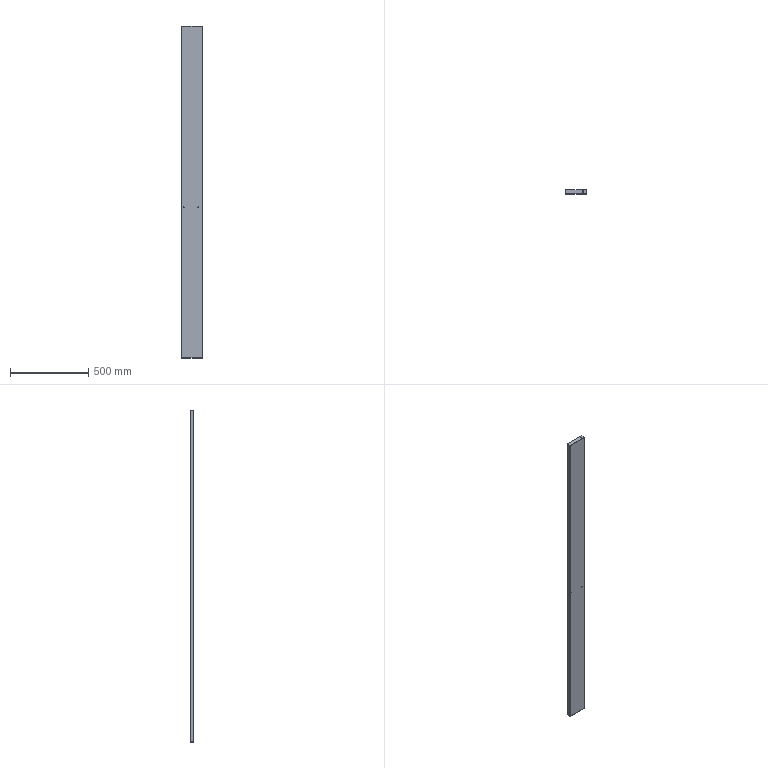Part | SolidWorks | features ICE 2, EdgeFlange 1, FlatPattern 1, HoleWzd 1, SMBaseFlange 1, SheetMetal 1 | 1 solid | 60 faces | box 132 x 25 x 2116 mm | volume 573342 mm3 | plane 30 | cylinder 22 | spline 8 | commonest cylinder face diameters 6.5 x10 0.6 x4 3.6 x4 4.2 x4